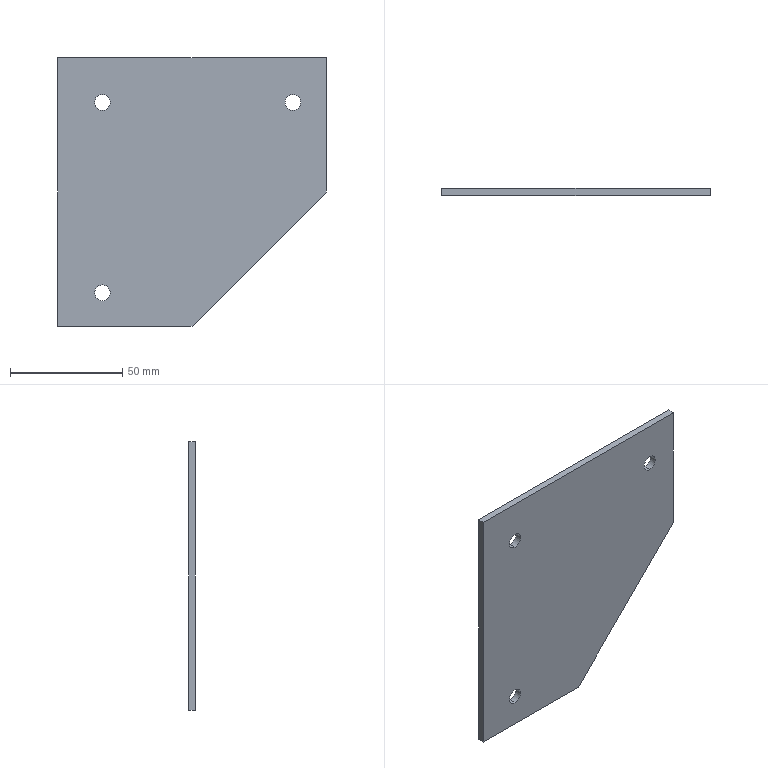Part | SolidWorks | features BaseBody 1 | 1 solid | 13 faces | box 120 x 3 x 120 mm | volume 37454 mm3 | plane 7 | cylinder 6 | commonest cylinder face diameters 7 x6
STEP:
#1=CARTESIAN_POINT('',(20.,0.,-108.5));
#2=VERTEX_POINT('',#1);
#3=CARTESIAN_POINT('',(20.,0.,-101.5));
#4=VERTEX_POINT('',#3);
#5=CARTESIAN_POINT('',(20.,0.,-105.));
#6=DIRECTION('',(0.,1.,0.));
#7=DIRECTION('',(0.,0.,-1.));
#8=AXIS2_PLACEMENT_3D('',#5,#6,#7);
#9=CIRCLE('',#8,3.5);
#10=EDGE_CURVE('',#2,#4,#9,.T.);
#11=ORIENTED_EDGE('',*,*,#10,.F.);
#12=CARTESIAN_POINT('',(20.,3.,-108.5));
#13=VERTEX_POINT('',#12);
#14=CARTESIAN_POINT('',(20.,0.,-108.5));
#15=DIRECTION('',(0.,1.,0.));
#16=VECTOR('',#15,1000.);
#17=LINE('',#14,#16);
#18=EDGE_CURVE('',#2,#13,#17,.T.);
#19=ORIENTED_EDGE('',*,*,#18,.T.);
#20=CARTESIAN_POINT('',(20.,3.,-101.5));
#21=VERTEX_POINT('',#20);
#22=CARTESIAN_POINT('',(20.,3.,-105.));
#23=DIRECTION('',(0.,1.,0.));
#24=DIRECTION('',(0.,0.,-1.));
#25=AXIS2_PLACEMENT_3D('',#22,#23,#24);
#26=CIRCLE('',#25,3.5);
#27=EDGE_CURVE('',#13,#21,#26,.T.);
#28=ORIENTED_EDGE('',*,*,#27,.T.);
#29=CARTESIAN_POINT('',(20.,0.,-101.5));
#30=DIRECTION('',(0.,1.,0.));
#31=VECTOR('',#30,1000.);
#32=LINE('',#29,#31);
#33=EDGE_CURVE('',#4,#21,#32,.T.);
#34=ORIENTED_EDGE('',*,*,#33,.F.);
#35=EDGE_LOOP('',(#11,#19,#28,#34));
#36=FACE_OUTER_BOUND('',#35,.T.);
#37=CARTESIAN_POINT('',(20.,0.,-105.));
#38=DIRECTION('',(0.,1.,0.));
#39=DIRECTION('',(0.,0.,1.));
#40=AXIS2_PLACEMENT_3D('',#37,#38,#39);
#41=CYLINDRICAL_SURFACE('',#40,3.5);
#42=ADVANCED_FACE('',(#36),#41,.F.);
#43=CARTESIAN_POINT('',(105.,0.,-23.5));
#44=VERTEX_POINT('',#43);
#45=CARTESIAN_POINT('',(105.,0.,-16.5));
#46=VERTEX_POINT('',#45);
#47=CARTESIAN_POINT('',(105.,0.,-20.));
#48=DIRECTION('',(0.,1.,0.));
#49=DIRECTION('',(0.,0.,1.));
#50=AXIS2_PLACEMENT_3D('',#47,#48,#49);
#51=CIRCLE('',#50,3.5);
#52=EDGE_CURVE('',#44,#46,#51,.T.);
#53=ORIENTED_EDGE('',*,*,#52,.F.);
#54=CARTESIAN_POINT('',(105.,3.,-23.5));
#55=VERTEX_POINT('',#54);
#56=CARTESIAN_POINT('',(105.,0.,-23.5));
#57=DIRECTION('',(0.,1.,0.));
#58=VECTOR('',#57,1000.);
#59=LINE('',#56,#58);
#60=EDGE_CURVE('',#44,#55,#59,.T.);
#61=ORIENTED_EDGE('',*,*,#60,.T.);
#62=CARTESIAN_POINT('',(105.,3.,-16.5));
#63=VERTEX_POINT('',#62);
#64=CARTESIAN_POINT('',(105.,3.,-20.));
#65=DIRECTION('',(0.,1.,0.));
#66=DIRECTION('',(0.,0.,1.));
#67=AXIS2_PLACEMENT_3D('',#64,#65,#66);
#68=CIRCLE('',#67,3.5);
#69=EDGE_CURVE('',#55,#63,#68,.T.);
#70=ORIENTED_EDGE('',*,*,#69,.T.);
#71=CARTESIAN_POINT('',(105.,0.,-16.5));
#72=DIRECTION('',(0.,1.,0.));
#73=VECTOR('',#72,1000.);
#74=LINE('',#71,#73);
#75=EDGE_CURVE('',#46,#63,#74,.T.);
#76=ORIENTED_EDGE('',*,*,#75,.F.);
#77=EDGE_LOOP('',(#53,#61,#70,#76));
#78=FACE_OUTER_BOUND('',#77,.T.);
#79=CARTESIAN_POINT('',(105.,0.,-20.));
#80=DIRECTION('',(0.,1.,0.));
#81=DIRECTION('',(0.,0.,1.));
#82=AXIS2_PLACEMENT_3D('',#79,#80,#81);
#83=CYLINDRICAL_SURFACE('',#82,3.5);
#84=ADVANCED_FACE('',(#78),#83,.F.);
#85=CARTESIAN_POINT('',(20.,0.,-23.5));
#86=VERTEX_POINT('',#85);
#87=CARTESIAN_POINT('',(20.,0.,-16.5));
#88=VERTEX_POINT('',#87);
#89=CARTESIAN_POINT('',(20.,0.,-20.));
#90=DIRECTION('',(0.,1.,0.));
#91=DIRECTION('',(0.,0.,1.));
#92=AXIS2_PLACEMENT_3D('',#89,#90,#91);
#93=CIRCLE('',#92,3.5);
#94=EDGE_CURVE('',#86,#88,#93,.T.);
#95=ORIENTED_EDGE('',*,*,#94,.F.);
#96=CARTESIAN_POINT('',(20.,3.,-23.5));
#97=VERTEX_POINT('',#96);
#98=CARTESIAN_POINT('',(20.,0.,-23.5));
#99=DIRECTION('',(0.,1.,0.));
#100=VECTOR('',#99,1000.);
#101=LINE('',#98,#100);
#102=EDGE_CURVE('',#86,#97,#101,.T.);
#103=ORIENTED_EDGE('',*,*,#102,.T.);
#104=CARTESIAN_POINT('',(20.,3.,-16.5));
#105=VERTEX_POINT('',#104);
#106=CARTESIAN_POINT('',(20.,3.,-20.));
#107=DIRECTION('',(0.,1.,0.));
#108=DIRECTION('',(0.,0.,1.));
#109=AXIS2_PLACEMENT_3D('',#106,#107,#108);
#110=CIRCLE('',#109,3.5);
#111=EDGE_CURVE('',#97,#105,#110,.T.);
#112=ORIENTED_EDGE('',*,*,#111,.T.);
#113=CARTESIAN_POINT('',(20.,0.,-16.5));
#114=DIRECTION('',(0.,1.,0.));
#115=VECTOR('',#114,1000.);
#116=LINE('',#113,#115);
#117=EDGE_CURVE('',#88,#105,#116,.T.);
#118=ORIENTED_EDGE('',*,*,#117,.F.);
#119=EDGE_LOOP('',(#95,#103,#112,#118));
#120=FACE_OUTER_BOUND('',#119,.T.);
#121=CARTESIAN_POINT('',(20.,0.,-20.));
#122=DIRECTION('',(0.,1.,0.));
#123=DIRECTION('',(0.,0.,1.));
#124=AXIS2_PLACEMENT_3D('',#121,#122,#123);
#125=CYLINDRICAL_SURFACE('',#124,3.5);
#126=ADVANCED_FACE('',(#120),#125,.F.);
#127=CARTESIAN_POINT('',(20.,0.,-20.));
#128=DIRECTION('',(0.,1.,0.));
#129=DIRECTION('',(0.,0.,1.));
#130=AXIS2_PLACEMENT_3D('',#127,#128,#129);
#131=CIRCLE('',#130,3.5);
#132=EDGE_CURVE('',#88,#86,#131,.T.);
#133=ORIENTED_EDGE('',*,*,#132,.T.);
#134=ORIENTED_EDGE('',*,*,#94,.T.);
#135=EDGE_LOOP('',(#133,#134));
#136=FACE_BOUND('',#135,.T.);
#137=CARTESIAN_POINT('',(105.,0.,-20.));
#138=DIRECTION('',(0.,1.,0.));
#139=DIRECTION('',(0.,0.,1.));
#140=AXIS2_PLACEMENT_3D('',#137,#138,#139);
#141=CIRCLE('',#140,3.5);
#142=EDGE_CURVE('',#46,#44,#141,.T.);
#143=ORIENTED_EDGE('',*,*,#142,.T.);
#144=ORIENTED_EDGE('',*,*,#52,.T.);
#145=EDGE_LOOP('',(#143,#144));
#146=FACE_BOUND('',#145,.T.);
#147=CARTESIAN_POINT('',(20.,0.,-105.));
#148=DIRECTION('',(0.,1.,0.));
#149=DIRECTION('',(0.,0.,-1.));
#150=AXIS2_PLACEMENT_3D('',#147,#148,#149);
#151=CIRCLE('',#150,3.5);
#152=EDGE_CURVE('',#4,#2,#151,.T.);
#153=ORIENTED_EDGE('',*,*,#152,.T.);
#154=ORIENTED_EDGE('',*,*,#10,.T.);
#155=EDGE_LOOP('',(#153,#154));
#156=FACE_BOUND('',#155,.T.);
#157=CARTESIAN_POINT('',(0.,0.,-120.));
#158=VERTEX_POINT('',#157);
#159=CARTESIAN_POINT('',(0.,0.,0.));
#160=VERTEX_POINT('',#159);
#161=CARTESIAN_POINT('',(0.,0.,0.));
#162=DIRECTION('',(0.,0.,1.));
#163=VECTOR('',#162,1000.);
#164=LINE('',#161,#163);
#165=EDGE_CURVE('',#158,#160,#164,.T.);
#166=ORIENTED_EDGE('',*,*,#165,.F.);
#167=CARTESIAN_POINT('',(60.,0.,-120.));
#168=VERTEX_POINT('',#167);
#169=CARTESIAN_POINT('',(0.,0.,-120.));
#170=DIRECTION('',(-1.,0.,0.));
#171=VECTOR('',#170,1000.);
#172=LINE('',#169,#171);
#173=EDGE_CURVE('',#168,#158,#172,.T.);
#174=ORIENTED_EDGE('',*,*,#173,.F.);
#175=CARTESIAN_POINT('',(120.,0.,-60.));
#176=VERTEX_POINT('',#175);
#177=CARTESIAN_POINT('',(60.,0.,-120.));
#178=DIRECTION('',(-0.7071,0.,-0.7071));
#179=VECTOR('',#178,1000.);
#180=LINE('',#177,#179);
#181=EDGE_CURVE('',#176,#168,#180,.T.);
#182=ORIENTED_EDGE('',*,*,#181,.F.);
#183=CARTESIAN_POINT('',(120.,0.,0.));
#184=VERTEX_POINT('',#183);
#185=CARTESIAN_POINT('',(120.,0.,0.));
#186=DIRECTION('',(0.,0.,-1.));
#187=VECTOR('',#186,1000.);
#188=LINE('',#185,#187);
#189=EDGE_CURVE('',#184,#176,#188,.T.);
#190=ORIENTED_EDGE('',*,*,#189,.F.);
#191=CARTESIAN_POINT('',(0.,0.,0.));
#192=DIRECTION('',(1.,0.,0.));
#193=VECTOR('',#192,1000.);
#194=LINE('',#191,#193);
#195=EDGE_CURVE('',#160,#184,#194,.T.);
#196=ORIENTED_EDGE('',*,*,#195,.F.);
#197=EDGE_LOOP('',(#166,#174,#182,#190,#196));
#198=FACE_OUTER_BOUND('',#197,.T.);
#199=CARTESIAN_POINT('',(0.,0.,0.));
#200=DIRECTION('',(0.,-1.,0.));
#201=DIRECTION('',(0.,0.,-1.));
#202=AXIS2_PLACEMENT_3D('',#199,#200,#201);
#203=PLANE('',#202);
#204=ADVANCED_FACE('',(#136,#146,#156,#198),#203,.T.);
#205=CARTESIAN_POINT('',(20.,3.,-20.));
#206=DIRECTION('',(0.,1.,0.));
#207=DIRECTION('',(0.,0.,1.));
#208=AXIS2_PLACEMENT_3D('',#205,#206,#207);
#209=CIRCLE('',#208,3.5);
#210=EDGE_CURVE('',#105,#97,#209,.T.);
#211=ORIENTED_EDGE('',*,*,#210,.F.);
#212=ORIENTED_EDGE('',*,*,#111,.F.);
#213=EDGE_LOOP('',(#211,#212));
#214=FACE_BOUND('',#213,.T.);
#215=CARTESIAN_POINT('',(105.,3.,-20.));
#216=DIRECTION('',(0.,1.,0.));
#217=DIRECTION('',(0.,0.,1.));
#218=AXIS2_PLACEMENT_3D('',#215,#216,#217);
#219=CIRCLE('',#218,3.5);
#220=EDGE_CURVE('',#63,#55,#219,.T.);
#221=ORIENTED_EDGE('',*,*,#220,.F.);
#222=ORIENTED_EDGE('',*,*,#69,.F.);
#223=EDGE_LOOP('',(#221,#222));
#224=FACE_BOUND('',#223,.T.);
#225=CARTESIAN_POINT('',(20.,3.,-105.));
#226=DIRECTION('',(0.,1.,0.));
#227=DIRECTION('',(0.,0.,-1.));
#228=AXIS2_PLACEMENT_3D('',#225,#226,#227);
#229=CIRCLE('',#228,3.5);
#230=EDGE_CURVE('',#21,#13,#229,.T.);
#231=ORIENTED_EDGE('',*,*,#230,.F.);
#232=ORIENTED_EDGE('',*,*,#27,.F.);
#233=EDGE_LOOP('',(#231,#232));
#234=FACE_BOUND('',#233,.T.);
#235=CARTESIAN_POINT('',(0.,3.,-120.));
#236=VERTEX_POINT('',#235);
#237=CARTESIAN_POINT('',(0.,3.,0.));
#238=VERTEX_POINT('',#237);
#239=CARTESIAN_POINT('',(0.,3.,0.));
#240=DIRECTION('',(0.,0.,1.));
#241=VECTOR('',#240,1000.);
#242=LINE('',#239,#241);
#243=EDGE_CURVE('',#236,#238,#242,.T.);
#244=ORIENTED_EDGE('',*,*,#243,.T.);
#245=CARTESIAN_POINT('',(120.,3.,0.));
#246=VERTEX_POINT('',#245);
#247=CARTESIAN_POINT('',(0.,3.,0.));
#248=DIRECTION('',(1.,0.,0.));
#249=VECTOR('',#248,1000.);
#250=LINE('',#247,#249);
#251=EDGE_CURVE('',#238,#246,#250,.T.);
#252=ORIENTED_EDGE('',*,*,#251,.T.);
#253=CARTESIAN_POINT('',(120.,3.,-60.));
#254=VERTEX_POINT('',#253);
#255=CARTESIAN_POINT('',(120.,3.,0.));
#256=DIRECTION('',(0.,0.,-1.));
#257=VECTOR('',#256,1000.);
#258=LINE('',#255,#257);
#259=EDGE_CURVE('',#246,#254,#258,.T.);
#260=ORIENTED_EDGE('',*,*,#259,.T.);
#261=CARTESIAN_POINT('',(60.,3.,-120.));
#262=VERTEX_POINT('',#261);
#263=CARTESIAN_POINT('',(60.,3.,-120.));
#264=DIRECTION('',(-0.7071,0.,-0.7071));
#265=VECTOR('',#264,1000.);
#266=LINE('',#263,#265);
#267=EDGE_CURVE('',#254,#262,#266,.T.);
#268=ORIENTED_EDGE('',*,*,#267,.T.);
#269=CARTESIAN_POINT('',(0.,3.,-120.));
#270=DIRECTION('',(-1.,0.,0.));
#271=VECTOR('',#270,1000.);
#272=LINE('',#269,#271);
#273=EDGE_CURVE('',#262,#236,#272,.T.);
#274=ORIENTED_EDGE('',*,*,#273,.T.);
#275=EDGE_LOOP('',(#244,#252,#260,#268,#274));
#276=FACE_OUTER_BOUND('',#275,.T.);
#277=CARTESIAN_POINT('',(0.,3.,0.));
#278=DIRECTION('',(0.,-1.,0.));
#279=DIRECTION('',(0.,0.,-1.));
#280=AXIS2_PLACEMENT_3D('',#277,#278,#279);
#281=PLANE('',#280);
#282=ADVANCED_FACE('',(#214,#224,#234,#276),#281,.F.);
#283=ORIENTED_EDGE('',*,*,#173,.T.);
#284=CARTESIAN_POINT('',(0.,3.,-120.));
#285=DIRECTION('',(0.,-1.,0.));
#286=VECTOR('',#285,1000.);
#287=LINE('',#284,#286);
#288=EDGE_CURVE('',#236,#158,#287,.T.);
#289=ORIENTED_EDGE('',*,*,#288,.F.);
#290=ORIENTED_EDGE('',*,*,#273,.F.);
#291=CARTESIAN_POINT('',(60.,3.,-120.));
#292=DIRECTION('',(0.,-1.,0.));
#293=VECTOR('',#292,1000.);
#294=LINE('',#291,#293);
#295=EDGE_CURVE('',#262,#168,#294,.T.);
#296=ORIENTED_EDGE('',*,*,#295,.T.);
#297=EDGE_LOOP('',(#283,#289,#290,#296));
#298=FACE_OUTER_BOUND('',#297,.T.);
#299=CARTESIAN_POINT('',(0.,3.,-120.));
#300=DIRECTION('',(0.,0.,1.));
#301=DIRECTION('',(1.,0.,0.));
#302=AXIS2_PLACEMENT_3D('',#299,#300,#301);
#303=PLANE('',#302);
#304=ADVANCED_FACE('',(#298),#303,.F.);
#305=ORIENTED_EDGE('',*,*,#181,.T.);
#306=ORIENTED_EDGE('',*,*,#295,.F.);
#307=ORIENTED_EDGE('',*,*,#267,.F.);
#308=CARTESIAN_POINT('',(120.,3.,-60.));
#309=DIRECTION('',(0.,-1.,0.));
#310=VECTOR('',#309,1000.);
#311=LINE('',#308,#310);
#312=EDGE_CURVE('',#254,#176,#311,.T.);
#313=ORIENTED_EDGE('',*,*,#312,.T.);
#314=EDGE_LOOP('',(#305,#306,#307,#313));
#315=FACE_OUTER_BOUND('',#314,.T.);
#316=CARTESIAN_POINT('',(60.,3.,-120.));
#317=DIRECTION('',(-0.7071,0.,0.7071));
#318=DIRECTION('',(0.,1.,0.));
#319=AXIS2_PLACEMENT_3D('',#316,#317,#318);
#320=PLANE('',#319);
#321=ADVANCED_FACE('',(#315),#320,.F.);
#322=ORIENTED_EDGE('',*,*,#189,.T.);
#323=ORIENTED_EDGE('',*,*,#312,.F.);
#324=ORIENTED_EDGE('',*,*,#259,.F.);
#325=CARTESIAN_POINT('',(120.,3.,0.));
#326=DIRECTION('',(0.,-1.,0.));
#327=VECTOR('',#326,1000.);
#328=LINE('',#325,#327);
#329=EDGE_CURVE('',#246,#184,#328,.T.);
#330=ORIENTED_EDGE('',*,*,#329,.T.);
#331=EDGE_LOOP('',(#322,#323,#324,#330));
#332=FACE_OUTER_BOUND('',#331,.T.);
#333=CARTESIAN_POINT('',(120.,3.,0.));
#334=DIRECTION('',(-1.,0.,0.));
#335=DIRECTION('',(0.,0.,1.));
#336=AXIS2_PLACEMENT_3D('',#333,#334,#335);
#337=PLANE('',#336);
#338=ADVANCED_FACE('',(#332),#337,.F.);
#339=ORIENTED_EDGE('',*,*,#195,.T.);
#340=ORIENTED_EDGE('',*,*,#329,.F.);
#341=ORIENTED_EDGE('',*,*,#251,.F.);
#342=CARTESIAN_POINT('',(0.,3.,0.));
#343=DIRECTION('',(0.,-1.,0.));
#344=VECTOR('',#343,1000.);
#345=LINE('',#342,#344);
#346=EDGE_CURVE('',#238,#160,#345,.T.);
#347=ORIENTED_EDGE('',*,*,#346,.T.);
#348=EDGE_LOOP('',(#339,#340,#341,#347));
#349=FACE_OUTER_BOUND('',#348,.T.);
#350=CARTESIAN_POINT('',(0.,3.,0.));
#351=DIRECTION('',(0.,0.,-1.));
#352=DIRECTION('',(0.,-1.,0.));
#353=AXIS2_PLACEMENT_3D('',#350,#351,#352);
#354=PLANE('',#353);
#355=ADVANCED_FACE('',(#349),#354,.F.);
#356=ORIENTED_EDGE('',*,*,#165,.T.);
#357=ORIENTED_EDGE('',*,*,#346,.F.);
#358=ORIENTED_EDGE('',*,*,#243,.F.);
#359=ORIENTED_EDGE('',*,*,#288,.T.);
#360=EDGE_LOOP('',(#356,#357,#358,#359));
#361=FACE_OUTER_BOUND('',#360,.T.);
#362=CARTESIAN_POINT('',(0.,3.,0.));
#363=DIRECTION('',(1.,0.,0.));
#364=DIRECTION('',(0.,1.,0.));
#365=AXIS2_PLACEMENT_3D('',#362,#363,#364);
#366=PLANE('',#365);
#367=ADVANCED_FACE('',(#361),#366,.F.);
#368=ORIENTED_EDGE('',*,*,#102,.F.);
#369=ORIENTED_EDGE('',*,*,#132,.F.);
#370=ORIENTED_EDGE('',*,*,#117,.T.);
#371=ORIENTED_EDGE('',*,*,#210,.T.);
#372=EDGE_LOOP('',(#368,#369,#370,#371));
#373=FACE_OUTER_BOUND('',#372,.T.);
#374=CARTESIAN_POINT('',(20.,0.,-20.));
#375=DIRECTION('',(0.,1.,0.));
#376=DIRECTION('',(0.,0.,1.));
#377=AXIS2_PLACEMENT_3D('',#374,#375,#376);
#378=CYLINDRICAL_SURFACE('',#377,3.5);
#379=ADVANCED_FACE('',(#373),#378,.F.);
#380=ORIENTED_EDGE('',*,*,#60,.F.);
#381=ORIENTED_EDGE('',*,*,#142,.F.);
#382=ORIENTED_EDGE('',*,*,#75,.T.);
#383=ORIENTED_EDGE('',*,*,#220,.T.);
#384=EDGE_LOOP('',(#380,#381,#382,#383));
#385=FACE_OUTER_BOUND('',#384,.T.);
#386=CARTESIAN_POINT('',(105.,0.,-20.));
#387=DIRECTION('',(0.,1.,0.));
#388=DIRECTION('',(0.,0.,1.));
#389=AXIS2_PLACEMENT_3D('',#386,#387,#388);
#390=CYLINDRICAL_SURFACE('',#389,3.5);
#391=ADVANCED_FACE('',(#385),#390,.F.);
#392=ORIENTED_EDGE('',*,*,#18,.F.);
#393=ORIENTED_EDGE('',*,*,#152,.F.);
#394=ORIENTED_EDGE('',*,*,#33,.T.);
#395=ORIENTED_EDGE('',*,*,#230,.T.);
#396=EDGE_LOOP('',(#392,#393,#394,#395));
#397=FACE_OUTER_BOUND('',#396,.T.);
#398=CARTESIAN_POINT('',(20.,0.,-105.));
#399=DIRECTION('',(0.,1.,0.));
#400=DIRECTION('',(0.,0.,1.));
#401=AXIS2_PLACEMENT_3D('',#398,#399,#400);
#402=CYLINDRICAL_SURFACE('',#401,3.5);
#403=ADVANCED_FACE('',(#397),#402,.F.);
#404=CLOSED_SHELL('',(#42,#84,#126,#204,#282,#304,#321,#338,#355,#367,#379,#391,#403));
#405=MANIFOLD_SOLID_BREP('',#404);
#406=CARTESIAN_POINT('',(0.,0.,0.));
#407=DIRECTION('',(0.,0.,1.));
#408=DIRECTION('',(1.,0.,0.));
#409=AXIS2_PLACEMENT_3D('',#406,#407,#408);
#410=(LENGTH_UNIT()NAMED_UNIT(*)SI_UNIT(.MILLI.,.METRE.));
#411=UNCERTAINTY_MEASURE_WITH_UNIT(LENGTH_MEASURE(0.00001),#410,'','');
#412=(NAMED_UNIT(*)PLANE_ANGLE_UNIT()SI_UNIT($,.RADIAN.));
#413=(NAMED_UNIT(*)SI_UNIT($,.STERADIAN.)SOLID_ANGLE_UNIT());
#414=(GEOMETRIC_REPRESENTATION_CONTEXT(3)GLOBAL_UNCERTAINTY_ASSIGNED_CONTEXT((#411))GLOBAL_UNIT_ASSIGNED_CONTEXT((#410,#412,#413))REPRESENTATION_CONTEXT('',''));
#415=ADVANCED_BREP_SHAPE_REPRESENTATION('',(#405,#409),#414);